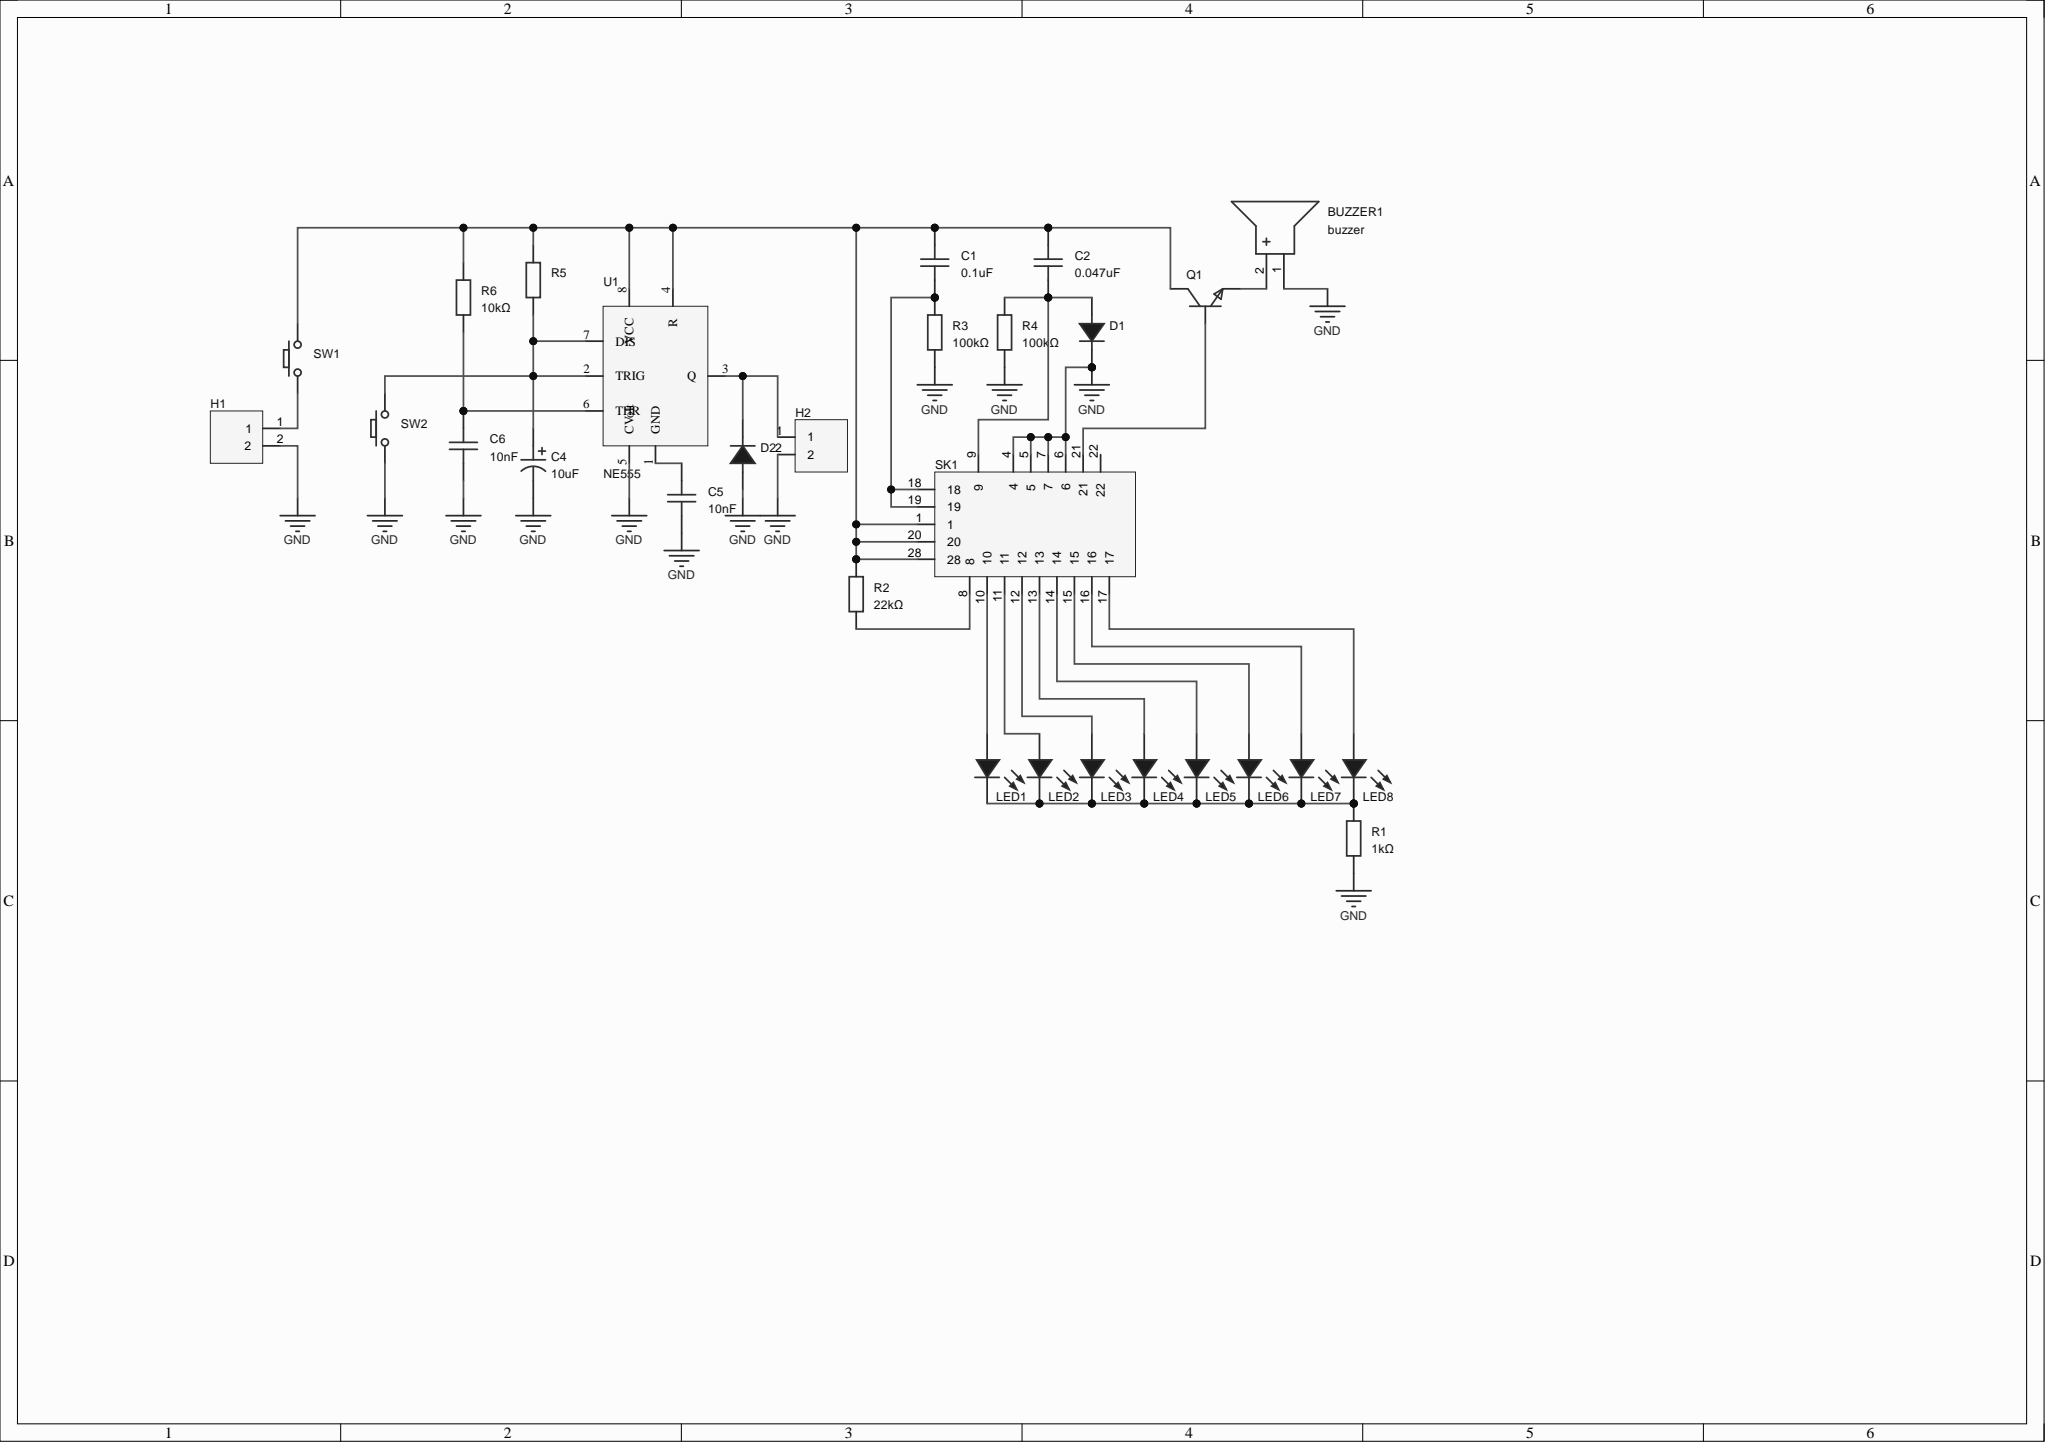Circuit board | Altium Designer | 29 parts | 21 nets
Bill of materials:
Comment,Description,Designator,Footprint,LibRef,Quantity
"buzzer","","BUZZER1","BUZ-TH_BD12.0-P6.00-D0.9-RD","buzzer","1"
"0.1uF","容值:100nF;精度:±10%;额定电压:50V;温度系数:X7R;","C1","CAP-TH_L5.1-W3.2-P5.08-D0.50","C323C104K5R5TA7301","1"
"0.047uF","容值:100nF;精度:±10%;额定电压:50V;温度系数:X7R;","C2","CAP-TH_L5.1-W3.2-P5.08-D0.50","C323C104K5R5TA7301","1"
"10uF","","C4","CAP-TH_BD5.0-P2.00-D0.8-FD-10UF50VC110GL","10UF50VC110GL","1"
"10nF","容值:100nF;精度:±10%;额定电压:50V;温度系数:X7R;","C5, C6","CAP-TH_L5.1-W3.2-P5.08-D0.50","C323C104K5R5TA7301","2"
"","","D1, D2","DO_1N4007","D_1N4007A","2"
"","","H1, H2","HDR-TH_2P-P2.54-V-M-1","HDR-M_2.54_1x2P","2"
"","","LED1, LED2, LED3, LED4, LED5, LED6, LED7, LED8","LED-TH_5mm","LED_TH-B_5mm","8"
"","","Q1","S8050_TO_92","S8050_TO_NPN","1"
"1kΩ","","R1","Res_1/8W","Res_AXIAL-1/8W","1"
"22kΩ","","R2","Res_1/8W","Res_AXIAL-1/8W","1"
"100kΩ","","R3, R4","Res_1/8W","Res_AXIAL-1/8W","2"
"10kΩ","","R5, R6","Res_1/8W","Res_AXIAL-1/8W","2"
"X5621WV-2x14-C762D1000-1000","适配封装类型:DIP;间距:2.54mm;行距:7.62mm;圆孔/方孔:圆孔;总PIN数:28P;工作温度:-40℃~+105℃;","SK1","DIP-28_L35.6-W10.2-P2.54-LS7.6-BL","X5621WV-2x14-C762D1000-1000","1"
"","","SW1, SW2","Key_TH_3.5x6x4.3","Key_TH_3.5x6x4.3","2"
"NE555","","U1","DIP-8_L9.8-W6.4-P2.54-LS7.6-BL","NE555","1"
Netlist (Protel format):
[
BUZZER1
BUZ-TH_BD12.0-P6.00-D0.9-RD
buzzer



]
[
C1
CAP-TH_L5.1-W3.2-P5.08-D0.50
0.1uF



]
[
C2
CAP-TH_L5.1-W3.2-P5.08-D0.50
0.047uF



]
[
C4
CAP-TH_BD5.0-P2.00-D0.8-FD-10UF50VC110GL
10uF



]
[
C5
CAP-TH_L5.1-W3.2-P5.08-D0.50
10nF



]
[
C6
CAP-TH_L5.1-W3.2-P5.08-D0.50
10nF



]
[
D1
DO_1N4007




]
[
D2
DO_1N4007




]
[
H1
HDR-TH_2P-P2.54-V-M-1




]
[
H2
HDR-TH_2P-P2.54-V-M-1




]
[
LED1
LED-TH_5mm




]
[
LED2
LED-TH_5mm




]
[
LED3
LED-TH_5mm




]
[
LED4
LED-TH_5mm




]
[
LED5
LED-TH_5mm




]
[
LED6
LED-TH_5mm




]
[
LED7
LED-TH_5mm




]
[
LED8
LED-TH_5mm




]
[
Q1
S8050_TO_92




]
[
R1
Res_1/8W
1kΩ



]
[
R2
Res_1/8W
22kΩ



]
[
R3
Res_1/8W
100kΩ



]
[
R4
Res_1/8W
100kΩ



]
[
R5
Res_1/8W
10kΩ



]
[
R6
Res_1/8W
10kΩ



]
[
SK1
DIP-28_L35.6-W10.2-P2.54-LS7.6-BL
X5621WV-2x14-C762D1000-1000



]
[
SW1
Key_TH_3.5x6x4.3




]
[
SW2
Key_TH_3.5x6x4.3




]
[
U1
DIP-8_L9.8-W6.4-P2.54-LS7.6-BL
NE555



]
(
NetR2_1
R2-1
SK1-8
)
(
NetQ1_2
Q1-2
SK1-21
)
(
NetLED8_1
LED8-1
SK1-17
)
(
NetLED7_1
LED7-1
SK1-16
)
(
NetLED6_1
LED6-1
SK1-15
)
(
NetLED5_1
LED5-1
SK1-14
)
(
NetLED4_1
LED4-1
SK1-13
)
(
NetLED3_1
LED3-1
SK1-12
)
(
NetLED2_1
LED2-1
SK1-11
)
(
NetLED1_2
LED1-2
LED2-2
LED3-2
LED4-2
LED5-2
LED6-2
LED7-2
LED8-2
R1-2
)
(
NetLED1_1
LED1-1
SK1-10
)
(
NetH1_1
H1-1
SW1-A
)
(
NetD2_1
D2-1
H2-1
U1-3
)
(
NetC6_2
C6-2
R6-1
U1-6
)
(
NetC5_2
C5-2
U1-1
)
(
NetC4_1
C4-1
R5-1
SW2-B
U1-2
U1-7
)
(
NetC2_1
C2-1
D1-2
R4-2
SK1-9
)
(
NetC1_2
C1-2
C2-2
Q1-3
R2-2
R5-2
R6-2
SK1-1
SK1-20
SK1-28
SW1-B
U1-4
U1-8
)
(
NetC1_1
C1-1
R3-2
SK1-18
SK1-19
)
(
NetBUZZER1_2
BUZZER1-2
Q1-1
)
(
GND
BUZZER1-1
C4-2
C5-1
C6-1
D1-1
D2-2
H1-2
H2-2
R1-1
R3-1
R4-1
SK1-4
SK1-5
SK1-6
SK1-7
SW2-A
U1-5
)